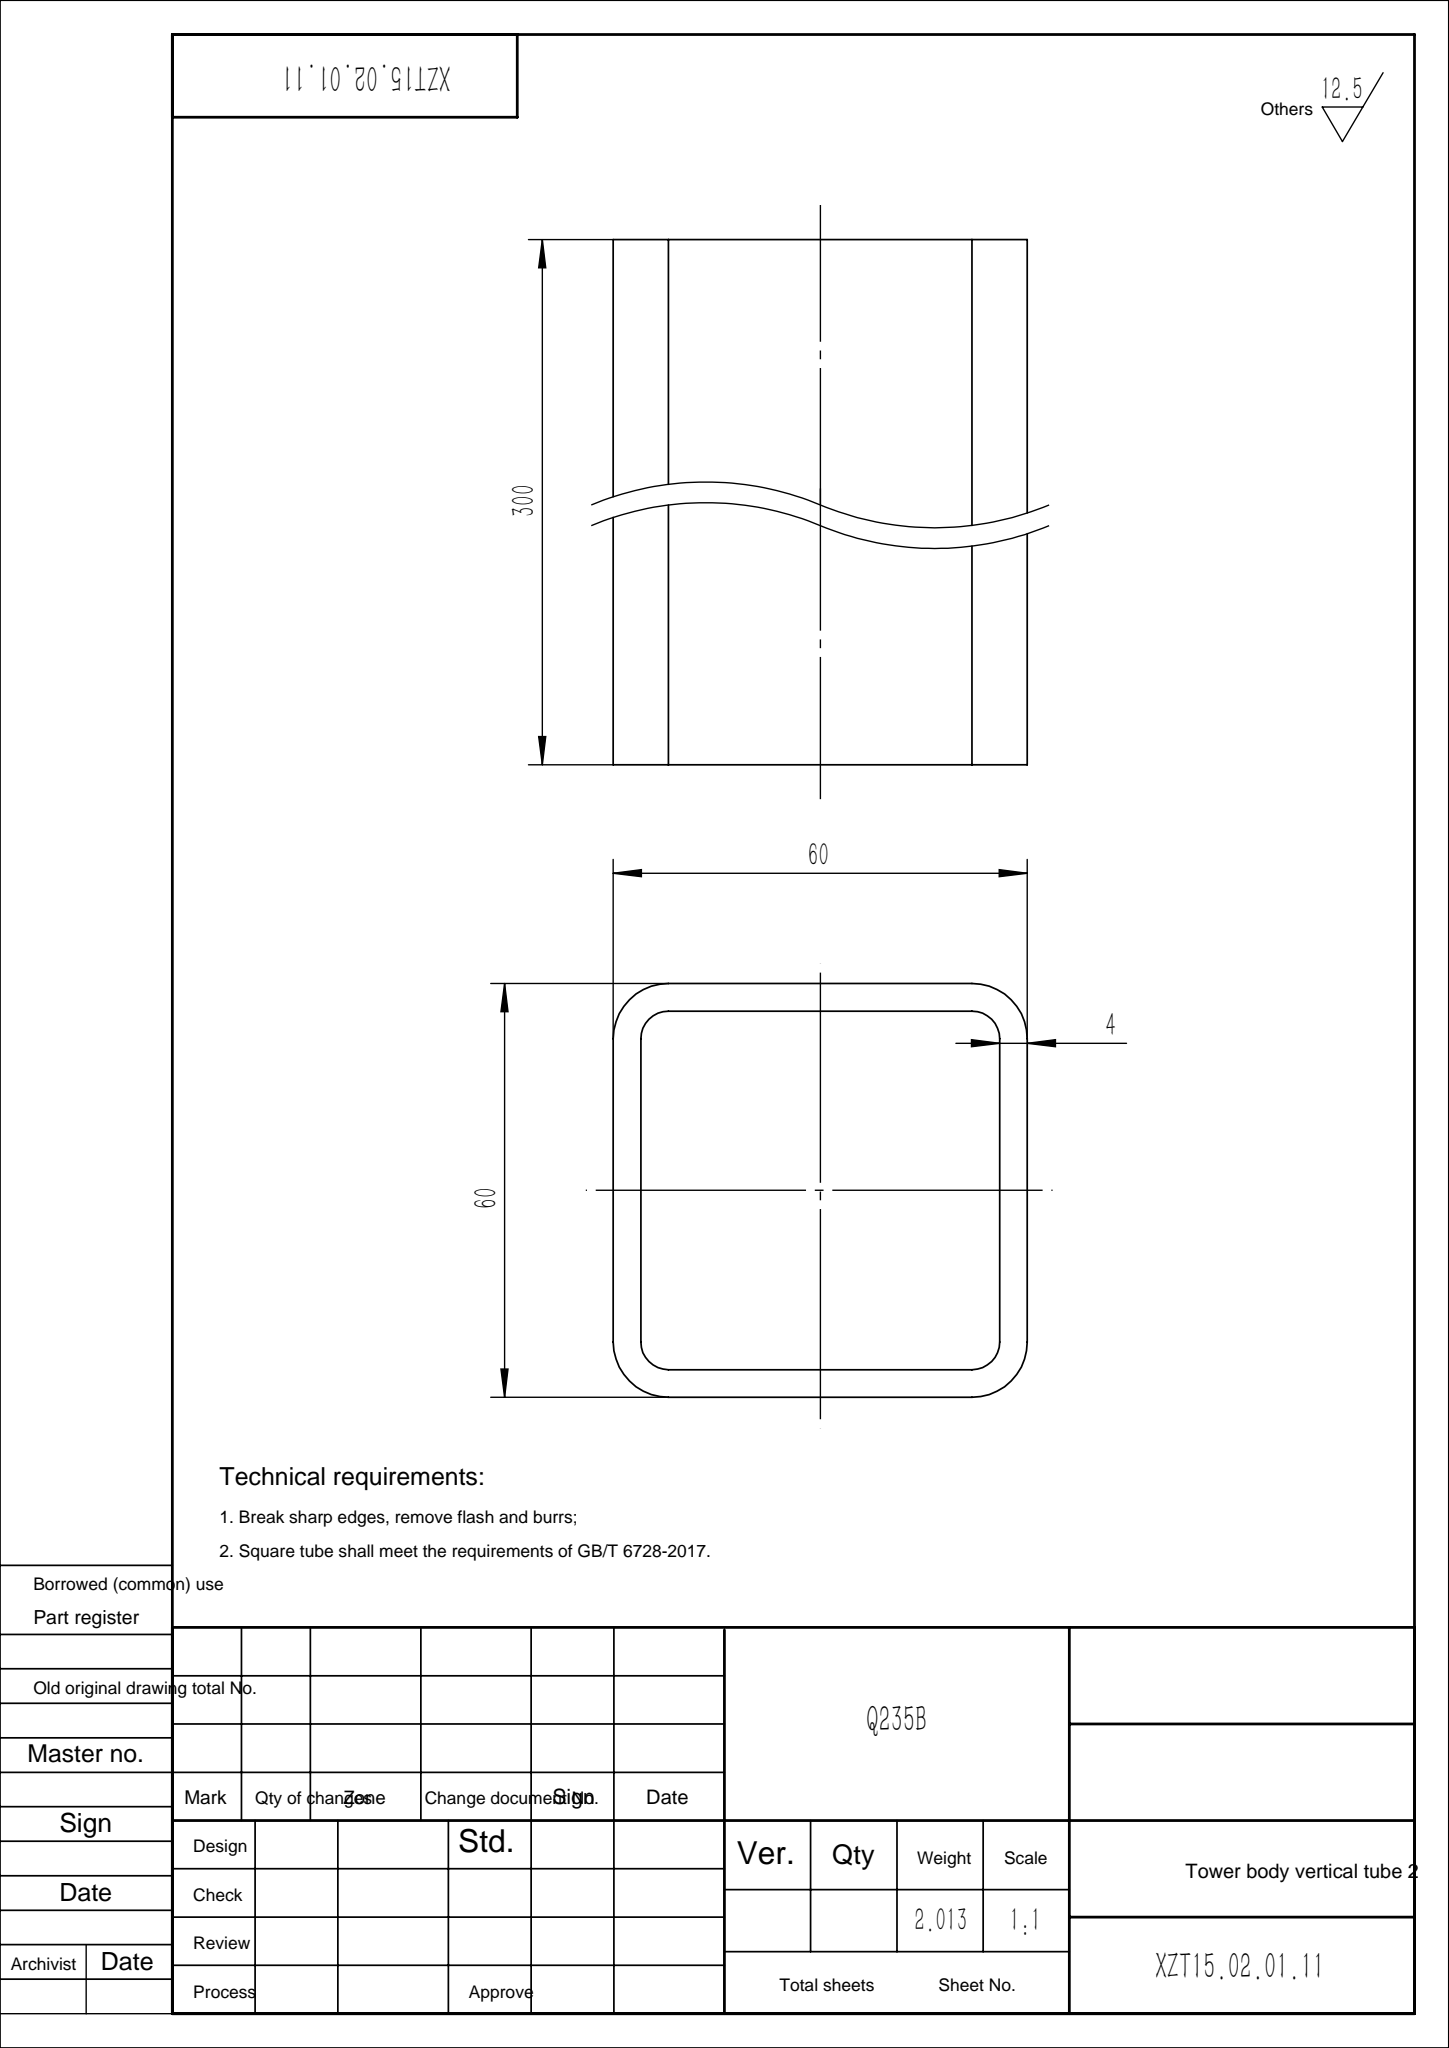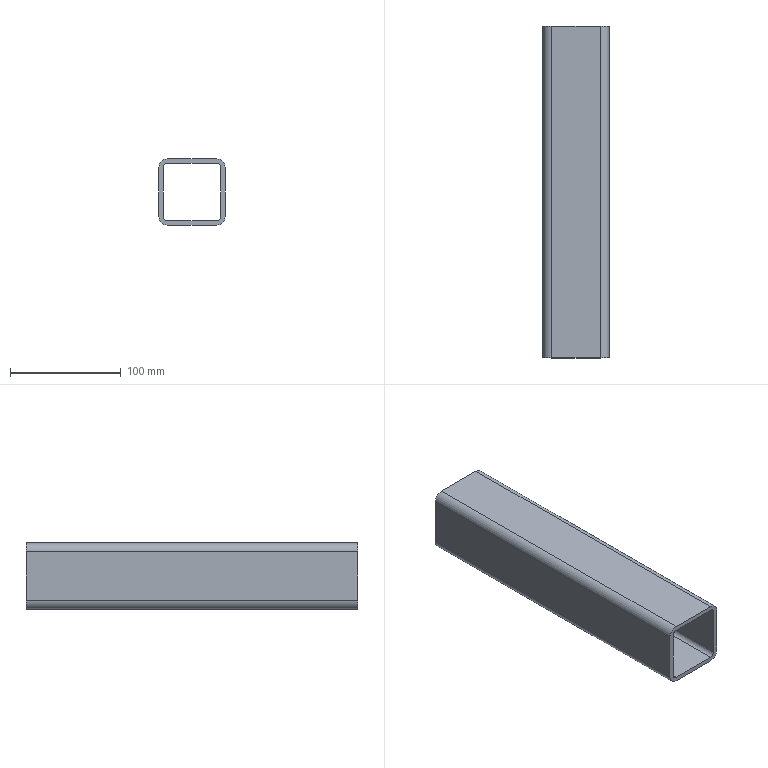Part | SolidWorks | features WeldMemberFeat 1, WeldmentFeature 1 | 1 solid | 18 faces | box 60 x 300 x 60 mm | volume 256439 mm3 | plane 10 | cylinder 8 | commonest cylinder face diameters 8 x4 16 x4
STEP:
#1=CARTESIAN_POINT('',(-30.,0.,22.));
#2=VERTEX_POINT('',#1);
#3=CARTESIAN_POINT('',(-22.,0.,30.));
#4=VERTEX_POINT('',#3);
#5=CARTESIAN_POINT('',(-22.,0.,22.));
#6=DIRECTION('',(0.,1.,0.));
#7=DIRECTION('',(0.,0.,1.));
#8=AXIS2_PLACEMENT_3D('',#5,#6,#7);
#9=CIRCLE('',#8,8.);
#10=EDGE_CURVE('',#2,#4,#9,.T.);
#11=ORIENTED_EDGE('',*,*,#10,.T.);
#12=CARTESIAN_POINT('',(-22.,300.,30.));
#13=VERTEX_POINT('',#12);
#14=CARTESIAN_POINT('',(-22.,300.,30.));
#15=DIRECTION('',(0.,-1.,0.));
#16=VECTOR('',#15,1000.);
#17=LINE('',#14,#16);
#18=EDGE_CURVE('',#13,#4,#17,.T.);
#19=ORIENTED_EDGE('',*,*,#18,.F.);
#20=CARTESIAN_POINT('',(-30.,300.,22.));
#21=VERTEX_POINT('',#20);
#22=CARTESIAN_POINT('',(-22.,300.,22.));
#23=DIRECTION('',(0.,1.,0.));
#24=DIRECTION('',(0.,0.,1.));
#25=AXIS2_PLACEMENT_3D('',#22,#23,#24);
#26=CIRCLE('',#25,8.);
#27=EDGE_CURVE('',#21,#13,#26,.T.);
#28=ORIENTED_EDGE('',*,*,#27,.F.);
#29=CARTESIAN_POINT('',(-30.,300.,22.));
#30=DIRECTION('',(0.,-1.,0.));
#31=VECTOR('',#30,1000.);
#32=LINE('',#29,#31);
#33=EDGE_CURVE('',#21,#2,#32,.T.);
#34=ORIENTED_EDGE('',*,*,#33,.T.);
#35=EDGE_LOOP('',(#11,#19,#28,#34));
#36=FACE_OUTER_BOUND('',#35,.T.);
#37=CARTESIAN_POINT('',(-22.,300.,22.));
#38=DIRECTION('',(0.,-1.,0.));
#39=DIRECTION('',(0.,0.,-1.));
#40=AXIS2_PLACEMENT_3D('',#37,#38,#39);
#41=CYLINDRICAL_SURFACE('',#40,8.);
#42=ADVANCED_FACE('',(#36),#41,.T.);
#43=CARTESIAN_POINT('',(22.,0.,30.));
#44=VERTEX_POINT('',#43);
#45=CARTESIAN_POINT('',(-22.,0.,30.));
#46=DIRECTION('',(1.,0.,0.));
#47=VECTOR('',#46,1000.);
#48=LINE('',#45,#47);
#49=EDGE_CURVE('',#4,#44,#48,.T.);
#50=ORIENTED_EDGE('',*,*,#49,.T.);
#51=CARTESIAN_POINT('',(22.,300.,30.));
#52=VERTEX_POINT('',#51);
#53=CARTESIAN_POINT('',(22.,300.,30.));
#54=DIRECTION('',(0.,-1.,0.));
#55=VECTOR('',#54,1000.);
#56=LINE('',#53,#55);
#57=EDGE_CURVE('',#52,#44,#56,.T.);
#58=ORIENTED_EDGE('',*,*,#57,.F.);
#59=CARTESIAN_POINT('',(-22.,300.,30.));
#60=DIRECTION('',(1.,0.,0.));
#61=VECTOR('',#60,1000.);
#62=LINE('',#59,#61);
#63=EDGE_CURVE('',#13,#52,#62,.T.);
#64=ORIENTED_EDGE('',*,*,#63,.F.);
#65=ORIENTED_EDGE('',*,*,#18,.T.);
#66=EDGE_LOOP('',(#50,#58,#64,#65));
#67=FACE_OUTER_BOUND('',#66,.T.);
#68=CARTESIAN_POINT('',(-22.,300.,30.));
#69=DIRECTION('',(0.,0.,-1.));
#70=DIRECTION('',(-1.,0.,0.));
#71=AXIS2_PLACEMENT_3D('',#68,#69,#70);
#72=PLANE('',#71);
#73=ADVANCED_FACE('',(#67),#72,.F.);
#74=CARTESIAN_POINT('',(30.,0.,22.));
#75=VERTEX_POINT('',#74);
#76=CARTESIAN_POINT('',(22.,0.,22.));
#77=DIRECTION('',(0.,1.,0.));
#78=DIRECTION('',(0.,0.,1.));
#79=AXIS2_PLACEMENT_3D('',#76,#77,#78);
#80=CIRCLE('',#79,8.);
#81=EDGE_CURVE('',#44,#75,#80,.T.);
#82=ORIENTED_EDGE('',*,*,#81,.T.);
#83=CARTESIAN_POINT('',(30.,300.,22.));
#84=VERTEX_POINT('',#83);
#85=CARTESIAN_POINT('',(30.,300.,22.));
#86=DIRECTION('',(0.,-1.,0.));
#87=VECTOR('',#86,1000.);
#88=LINE('',#85,#87);
#89=EDGE_CURVE('',#84,#75,#88,.T.);
#90=ORIENTED_EDGE('',*,*,#89,.F.);
#91=CARTESIAN_POINT('',(22.,300.,22.));
#92=DIRECTION('',(0.,1.,0.));
#93=DIRECTION('',(0.,0.,1.));
#94=AXIS2_PLACEMENT_3D('',#91,#92,#93);
#95=CIRCLE('',#94,8.);
#96=EDGE_CURVE('',#52,#84,#95,.T.);
#97=ORIENTED_EDGE('',*,*,#96,.F.);
#98=ORIENTED_EDGE('',*,*,#57,.T.);
#99=EDGE_LOOP('',(#82,#90,#97,#98));
#100=FACE_OUTER_BOUND('',#99,.T.);
#101=CARTESIAN_POINT('',(22.,300.,22.));
#102=DIRECTION('',(0.,-1.,0.));
#103=DIRECTION('',(0.,0.,-1.));
#104=AXIS2_PLACEMENT_3D('',#101,#102,#103);
#105=CYLINDRICAL_SURFACE('',#104,8.);
#106=ADVANCED_FACE('',(#100),#105,.T.);
#107=CARTESIAN_POINT('',(30.,0.,-22.));
#108=VERTEX_POINT('',#107);
#109=CARTESIAN_POINT('',(30.,0.,-22.));
#110=DIRECTION('',(0.,0.,-1.));
#111=VECTOR('',#110,1000.);
#112=LINE('',#109,#111);
#113=EDGE_CURVE('',#75,#108,#112,.T.);
#114=ORIENTED_EDGE('',*,*,#113,.T.);
#115=CARTESIAN_POINT('',(30.,300.,-22.));
#116=VERTEX_POINT('',#115);
#117=CARTESIAN_POINT('',(30.,300.,-22.));
#118=DIRECTION('',(0.,-1.,0.));
#119=VECTOR('',#118,1000.);
#120=LINE('',#117,#119);
#121=EDGE_CURVE('',#116,#108,#120,.T.);
#122=ORIENTED_EDGE('',*,*,#121,.F.);
#123=CARTESIAN_POINT('',(30.,300.,-22.));
#124=DIRECTION('',(0.,0.,-1.));
#125=VECTOR('',#124,1000.);
#126=LINE('',#123,#125);
#127=EDGE_CURVE('',#84,#116,#126,.T.);
#128=ORIENTED_EDGE('',*,*,#127,.F.);
#129=ORIENTED_EDGE('',*,*,#89,.T.);
#130=EDGE_LOOP('',(#114,#122,#128,#129));
#131=FACE_OUTER_BOUND('',#130,.T.);
#132=CARTESIAN_POINT('',(30.,300.,-22.));
#133=DIRECTION('',(-1.,0.,0.));
#134=DIRECTION('',(0.,0.,1.));
#135=AXIS2_PLACEMENT_3D('',#132,#133,#134);
#136=PLANE('',#135);
#137=ADVANCED_FACE('',(#131),#136,.F.);
#138=CARTESIAN_POINT('',(22.,0.,-30.));
#139=VERTEX_POINT('',#138);
#140=CARTESIAN_POINT('',(22.,0.,-22.));
#141=DIRECTION('',(0.,1.,0.));
#142=DIRECTION('',(0.,0.,1.));
#143=AXIS2_PLACEMENT_3D('',#140,#141,#142);
#144=CIRCLE('',#143,8.);
#145=EDGE_CURVE('',#108,#139,#144,.T.);
#146=ORIENTED_EDGE('',*,*,#145,.T.);
#147=CARTESIAN_POINT('',(22.,300.,-30.));
#148=VERTEX_POINT('',#147);
#149=CARTESIAN_POINT('',(22.,300.,-30.));
#150=DIRECTION('',(0.,-1.,0.));
#151=VECTOR('',#150,1000.);
#152=LINE('',#149,#151);
#153=EDGE_CURVE('',#148,#139,#152,.T.);
#154=ORIENTED_EDGE('',*,*,#153,.F.);
#155=CARTESIAN_POINT('',(22.,300.,-22.));
#156=DIRECTION('',(0.,1.,0.));
#157=DIRECTION('',(0.,0.,1.));
#158=AXIS2_PLACEMENT_3D('',#155,#156,#157);
#159=CIRCLE('',#158,8.);
#160=EDGE_CURVE('',#116,#148,#159,.T.);
#161=ORIENTED_EDGE('',*,*,#160,.F.);
#162=ORIENTED_EDGE('',*,*,#121,.T.);
#163=EDGE_LOOP('',(#146,#154,#161,#162));
#164=FACE_OUTER_BOUND('',#163,.T.);
#165=CARTESIAN_POINT('',(22.,300.,-22.));
#166=DIRECTION('',(0.,-1.,0.));
#167=DIRECTION('',(0.,0.,-1.));
#168=AXIS2_PLACEMENT_3D('',#165,#166,#167);
#169=CYLINDRICAL_SURFACE('',#168,8.);
#170=ADVANCED_FACE('',(#164),#169,.T.);
#171=CARTESIAN_POINT('',(-22.,0.,-30.));
#172=VERTEX_POINT('',#171);
#173=CARTESIAN_POINT('',(22.,0.,-30.));
#174=DIRECTION('',(-1.,0.,0.));
#175=VECTOR('',#174,1000.);
#176=LINE('',#173,#175);
#177=EDGE_CURVE('',#139,#172,#176,.T.);
#178=ORIENTED_EDGE('',*,*,#177,.T.);
#179=CARTESIAN_POINT('',(-22.,300.,-30.));
#180=VERTEX_POINT('',#179);
#181=CARTESIAN_POINT('',(-22.,300.,-30.));
#182=DIRECTION('',(0.,-1.,0.));
#183=VECTOR('',#182,1000.);
#184=LINE('',#181,#183);
#185=EDGE_CURVE('',#180,#172,#184,.T.);
#186=ORIENTED_EDGE('',*,*,#185,.F.);
#187=CARTESIAN_POINT('',(22.,300.,-30.));
#188=DIRECTION('',(-1.,0.,0.));
#189=VECTOR('',#188,1000.);
#190=LINE('',#187,#189);
#191=EDGE_CURVE('',#148,#180,#190,.T.);
#192=ORIENTED_EDGE('',*,*,#191,.F.);
#193=ORIENTED_EDGE('',*,*,#153,.T.);
#194=EDGE_LOOP('',(#178,#186,#192,#193));
#195=FACE_OUTER_BOUND('',#194,.T.);
#196=CARTESIAN_POINT('',(22.,300.,-30.));
#197=DIRECTION('',(0.,0.,1.));
#198=DIRECTION('',(1.,0.,0.));
#199=AXIS2_PLACEMENT_3D('',#196,#197,#198);
#200=PLANE('',#199);
#201=ADVANCED_FACE('',(#195),#200,.F.);
#202=CARTESIAN_POINT('',(-30.,0.,-22.));
#203=VERTEX_POINT('',#202);
#204=CARTESIAN_POINT('',(-22.,0.,-22.));
#205=DIRECTION('',(0.,1.,0.));
#206=DIRECTION('',(0.,0.,1.));
#207=AXIS2_PLACEMENT_3D('',#204,#205,#206);
#208=CIRCLE('',#207,8.);
#209=EDGE_CURVE('',#172,#203,#208,.T.);
#210=ORIENTED_EDGE('',*,*,#209,.T.);
#211=CARTESIAN_POINT('',(-30.,300.,-22.));
#212=VERTEX_POINT('',#211);
#213=CARTESIAN_POINT('',(-30.,300.,-22.));
#214=DIRECTION('',(0.,-1.,0.));
#215=VECTOR('',#214,1000.);
#216=LINE('',#213,#215);
#217=EDGE_CURVE('',#212,#203,#216,.T.);
#218=ORIENTED_EDGE('',*,*,#217,.F.);
#219=CARTESIAN_POINT('',(-22.,300.,-22.));
#220=DIRECTION('',(0.,1.,0.));
#221=DIRECTION('',(0.,0.,1.));
#222=AXIS2_PLACEMENT_3D('',#219,#220,#221);
#223=CIRCLE('',#222,8.);
#224=EDGE_CURVE('',#180,#212,#223,.T.);
#225=ORIENTED_EDGE('',*,*,#224,.F.);
#226=ORIENTED_EDGE('',*,*,#185,.T.);
#227=EDGE_LOOP('',(#210,#218,#225,#226));
#228=FACE_OUTER_BOUND('',#227,.T.);
#229=CARTESIAN_POINT('',(-22.,300.,-22.));
#230=DIRECTION('',(0.,-1.,0.));
#231=DIRECTION('',(0.,0.,-1.));
#232=AXIS2_PLACEMENT_3D('',#229,#230,#231);
#233=CYLINDRICAL_SURFACE('',#232,8.);
#234=ADVANCED_FACE('',(#228),#233,.T.);
#235=CARTESIAN_POINT('',(22.,0.,26.));
#236=VERTEX_POINT('',#235);
#237=CARTESIAN_POINT('',(26.,0.,22.));
#238=VERTEX_POINT('',#237);
#239=CARTESIAN_POINT('',(22.,0.,22.));
#240=DIRECTION('',(0.,1.,0.));
#241=DIRECTION('',(0.,0.,1.));
#242=AXIS2_PLACEMENT_3D('',#239,#240,#241);
#243=CIRCLE('',#242,4.);
#244=EDGE_CURVE('',#236,#238,#243,.T.);
#245=ORIENTED_EDGE('',*,*,#244,.F.);
#246=CARTESIAN_POINT('',(22.,300.,26.));
#247=VERTEX_POINT('',#246);
#248=CARTESIAN_POINT('',(22.,300.,26.));
#249=DIRECTION('',(0.,-1.,0.));
#250=VECTOR('',#249,1000.);
#251=LINE('',#248,#250);
#252=EDGE_CURVE('',#247,#236,#251,.T.);
#253=ORIENTED_EDGE('',*,*,#252,.F.);
#254=CARTESIAN_POINT('',(26.,300.,22.));
#255=VERTEX_POINT('',#254);
#256=CARTESIAN_POINT('',(22.,300.,22.));
#257=DIRECTION('',(0.,1.,0.));
#258=DIRECTION('',(0.,0.,1.));
#259=AXIS2_PLACEMENT_3D('',#256,#257,#258);
#260=CIRCLE('',#259,4.);
#261=EDGE_CURVE('',#247,#255,#260,.T.);
#262=ORIENTED_EDGE('',*,*,#261,.T.);
#263=CARTESIAN_POINT('',(26.,300.,22.));
#264=DIRECTION('',(0.,-1.,0.));
#265=VECTOR('',#264,1000.);
#266=LINE('',#263,#265);
#267=EDGE_CURVE('',#255,#238,#266,.T.);
#268=ORIENTED_EDGE('',*,*,#267,.T.);
#269=EDGE_LOOP('',(#245,#253,#262,#268));
#270=FACE_OUTER_BOUND('',#269,.T.);
#271=CARTESIAN_POINT('',(22.,300.,22.));
#272=DIRECTION('',(0.,-1.,0.));
#273=DIRECTION('',(0.,0.,-1.));
#274=AXIS2_PLACEMENT_3D('',#271,#272,#273);
#275=CYLINDRICAL_SURFACE('',#274,4.);
#276=ADVANCED_FACE('',(#270),#275,.F.);
#277=CARTESIAN_POINT('',(-22.,0.,26.));
#278=VERTEX_POINT('',#277);
#279=CARTESIAN_POINT('',(-22.,0.,26.));
#280=DIRECTION('',(1.,0.,0.));
#281=VECTOR('',#280,1000.);
#282=LINE('',#279,#281);
#283=EDGE_CURVE('',#278,#236,#282,.T.);
#284=ORIENTED_EDGE('',*,*,#283,.F.);
#285=CARTESIAN_POINT('',(-22.,300.,26.));
#286=VERTEX_POINT('',#285);
#287=CARTESIAN_POINT('',(-22.,300.,26.));
#288=DIRECTION('',(0.,-1.,0.));
#289=VECTOR('',#288,1000.);
#290=LINE('',#287,#289);
#291=EDGE_CURVE('',#286,#278,#290,.T.);
#292=ORIENTED_EDGE('',*,*,#291,.F.);
#293=CARTESIAN_POINT('',(-22.,300.,26.));
#294=DIRECTION('',(1.,0.,0.));
#295=VECTOR('',#294,1000.);
#296=LINE('',#293,#295);
#297=EDGE_CURVE('',#286,#247,#296,.T.);
#298=ORIENTED_EDGE('',*,*,#297,.T.);
#299=ORIENTED_EDGE('',*,*,#252,.T.);
#300=EDGE_LOOP('',(#284,#292,#298,#299));
#301=FACE_OUTER_BOUND('',#300,.T.);
#302=CARTESIAN_POINT('',(-22.,300.,26.));
#303=DIRECTION('',(0.,0.,-1.));
#304=DIRECTION('',(-1.,0.,0.));
#305=AXIS2_PLACEMENT_3D('',#302,#303,#304);
#306=PLANE('',#305);
#307=ADVANCED_FACE('',(#301),#306,.T.);
#308=CARTESIAN_POINT('',(-26.,0.,22.));
#309=VERTEX_POINT('',#308);
#310=CARTESIAN_POINT('',(-22.,0.,22.));
#311=DIRECTION('',(0.,1.,0.));
#312=DIRECTION('',(0.,0.,1.));
#313=AXIS2_PLACEMENT_3D('',#310,#311,#312);
#314=CIRCLE('',#313,4.);
#315=EDGE_CURVE('',#309,#278,#314,.T.);
#316=ORIENTED_EDGE('',*,*,#315,.F.);
#317=CARTESIAN_POINT('',(-26.,300.,22.));
#318=VERTEX_POINT('',#317);
#319=CARTESIAN_POINT('',(-26.,300.,22.));
#320=DIRECTION('',(0.,-1.,0.));
#321=VECTOR('',#320,1000.);
#322=LINE('',#319,#321);
#323=EDGE_CURVE('',#318,#309,#322,.T.);
#324=ORIENTED_EDGE('',*,*,#323,.F.);
#325=CARTESIAN_POINT('',(-22.,300.,22.));
#326=DIRECTION('',(0.,1.,0.));
#327=DIRECTION('',(0.,0.,1.));
#328=AXIS2_PLACEMENT_3D('',#325,#326,#327);
#329=CIRCLE('',#328,4.);
#330=EDGE_CURVE('',#318,#286,#329,.T.);
#331=ORIENTED_EDGE('',*,*,#330,.T.);
#332=ORIENTED_EDGE('',*,*,#291,.T.);
#333=EDGE_LOOP('',(#316,#324,#331,#332));
#334=FACE_OUTER_BOUND('',#333,.T.);
#335=CARTESIAN_POINT('',(-22.,300.,22.));
#336=DIRECTION('',(0.,-1.,0.));
#337=DIRECTION('',(0.,0.,-1.));
#338=AXIS2_PLACEMENT_3D('',#335,#336,#337);
#339=CYLINDRICAL_SURFACE('',#338,4.);
#340=ADVANCED_FACE('',(#334),#339,.F.);
#341=CARTESIAN_POINT('',(-26.,0.,-22.));
#342=VERTEX_POINT('',#341);
#343=CARTESIAN_POINT('',(-26.,0.,22.));
#344=DIRECTION('',(0.,0.,1.));
#345=VECTOR('',#344,1000.);
#346=LINE('',#343,#345);
#347=EDGE_CURVE('',#342,#309,#346,.T.);
#348=ORIENTED_EDGE('',*,*,#347,.F.);
#349=CARTESIAN_POINT('',(-26.,300.,-22.));
#350=VERTEX_POINT('',#349);
#351=CARTESIAN_POINT('',(-26.,300.,-22.));
#352=DIRECTION('',(0.,-1.,0.));
#353=VECTOR('',#352,1000.);
#354=LINE('',#351,#353);
#355=EDGE_CURVE('',#350,#342,#354,.T.);
#356=ORIENTED_EDGE('',*,*,#355,.F.);
#357=CARTESIAN_POINT('',(-26.,300.,22.));
#358=DIRECTION('',(0.,0.,1.));
#359=VECTOR('',#358,1000.);
#360=LINE('',#357,#359);
#361=EDGE_CURVE('',#350,#318,#360,.T.);
#362=ORIENTED_EDGE('',*,*,#361,.T.);
#363=ORIENTED_EDGE('',*,*,#323,.T.);
#364=EDGE_LOOP('',(#348,#356,#362,#363));
#365=FACE_OUTER_BOUND('',#364,.T.);
#366=CARTESIAN_POINT('',(-26.,300.,22.));
#367=DIRECTION('',(1.,0.,0.));
#368=DIRECTION('',(0.,0.,-1.));
#369=AXIS2_PLACEMENT_3D('',#366,#367,#368);
#370=PLANE('',#369);
#371=ADVANCED_FACE('',(#365),#370,.T.);
#372=CARTESIAN_POINT('',(-22.,0.,-26.));
#373=VERTEX_POINT('',#372);
#374=CARTESIAN_POINT('',(-22.,0.,-22.));
#375=DIRECTION('',(0.,1.,0.));
#376=DIRECTION('',(0.,0.,1.));
#377=AXIS2_PLACEMENT_3D('',#374,#375,#376);
#378=CIRCLE('',#377,4.);
#379=EDGE_CURVE('',#373,#342,#378,.T.);
#380=ORIENTED_EDGE('',*,*,#379,.F.);
#381=CARTESIAN_POINT('',(-22.,300.,-26.));
#382=VERTEX_POINT('',#381);
#383=CARTESIAN_POINT('',(-22.,300.,-26.));
#384=DIRECTION('',(0.,-1.,0.));
#385=VECTOR('',#384,1000.);
#386=LINE('',#383,#385);
#387=EDGE_CURVE('',#382,#373,#386,.T.);
#388=ORIENTED_EDGE('',*,*,#387,.F.);
#389=CARTESIAN_POINT('',(-22.,300.,-22.));
#390=DIRECTION('',(0.,1.,0.));
#391=DIRECTION('',(0.,0.,1.));
#392=AXIS2_PLACEMENT_3D('',#389,#390,#391);
#393=CIRCLE('',#392,4.);
#394=EDGE_CURVE('',#382,#350,#393,.T.);
#395=ORIENTED_EDGE('',*,*,#394,.T.);
#396=ORIENTED_EDGE('',*,*,#355,.T.);
#397=EDGE_LOOP('',(#380,#388,#395,#396));
#398=FACE_OUTER_BOUND('',#397,.T.);
#399=CARTESIAN_POINT('',(-22.,300.,-22.));
#400=DIRECTION('',(0.,-1.,0.));
#401=DIRECTION('',(0.,0.,-1.));
#402=AXIS2_PLACEMENT_3D('',#399,#400,#401);
#403=CYLINDRICAL_SURFACE('',#402,4.);
#404=ADVANCED_FACE('',(#398),#403,.F.);
#405=CARTESIAN_POINT('',(22.,0.,-26.));
#406=VERTEX_POINT('',#405);
#407=CARTESIAN_POINT('',(22.,0.,-26.));
#408=DIRECTION('',(-1.,0.,0.));
#409=VECTOR('',#408,1000.);
#410=LINE('',#407,#409);
#411=EDGE_CURVE('',#406,#373,#410,.T.);
#412=ORIENTED_EDGE('',*,*,#411,.F.);
#413=CARTESIAN_POINT('',(22.,300.,-26.));
#414=VERTEX_POINT('',#413);
#415=CARTESIAN_POINT('',(22.,300.,-26.));
#416=DIRECTION('',(0.,-1.,0.));
#417=VECTOR('',#416,1000.);
#418=LINE('',#415,#417);
#419=EDGE_CURVE('',#414,#406,#418,.T.);
#420=ORIENTED_EDGE('',*,*,#419,.F.);
#421=CARTESIAN_POINT('',(22.,300.,-26.));
#422=DIRECTION('',(-1.,0.,0.));
#423=VECTOR('',#422,1000.);
#424=LINE('',#421,#423);
#425=EDGE_CURVE('',#414,#382,#424,.T.);
#426=ORIENTED_EDGE('',*,*,#425,.T.);
#427=ORIENTED_EDGE('',*,*,#387,.T.);
#428=EDGE_LOOP('',(#412,#420,#426,#427));
#429=FACE_OUTER_BOUND('',#428,.T.);
#430=CARTESIAN_POINT('',(22.,300.,-26.));
#431=DIRECTION('',(0.,0.,1.));
#432=DIRECTION('',(1.,0.,0.));
#433=AXIS2_PLACEMENT_3D('',#430,#431,#432);
#434=PLANE('',#433);
#435=ADVANCED_FACE('',(#429),#434,.T.);
#436=CARTESIAN_POINT('',(26.,0.,-22.));
#437=VERTEX_POINT('',#436);
#438=CARTESIAN_POINT('',(22.,0.,-22.));
#439=DIRECTION('',(0.,1.,0.));
#440=DIRECTION('',(0.,0.,1.));
#441=AXIS2_PLACEMENT_3D('',#438,#439,#440);
#442=CIRCLE('',#441,4.);
#443=EDGE_CURVE('',#437,#406,#442,.T.);
#444=ORIENTED_EDGE('',*,*,#443,.F.);
#445=CARTESIAN_POINT('',(26.,300.,-22.));
#446=VERTEX_POINT('',#445);
#447=CARTESIAN_POINT('',(26.,300.,-22.));
#448=DIRECTION('',(0.,-1.,0.));
#449=VECTOR('',#448,1000.);
#450=LINE('',#447,#449);
#451=EDGE_CURVE('',#446,#437,#450,.T.);
#452=ORIENTED_EDGE('',*,*,#451,.F.);
#453=CARTESIAN_POINT('',(22.,300.,-22.));
#454=DIRECTION('',(0.,1.,0.));
#455=DIRECTION('',(0.,0.,1.));
#456=AXIS2_PLACEMENT_3D('',#453,#454,#455);
#457=CIRCLE('',#456,4.);
#458=EDGE_CURVE('',#446,#414,#457,.T.);
#459=ORIENTED_EDGE('',*,*,#458,.T.);
#460=ORIENTED_EDGE('',*,*,#419,.T.);
#461=EDGE_LOOP('',(#444,#452,#459,#460));
#462=FACE_OUTER_BOUND('',#461,.T.);
#463=CARTESIAN_POINT('',(22.,300.,-22.));
#464=DIRECTION('',(0.,-1.,0.));
#465=DIRECTION('',(0.,0.,-1.));
#466=AXIS2_PLACEMENT_3D('',#463,#464,#465);
#467=CYLINDRICAL_SURFACE('',#466,4.);
#468=ADVANCED_FACE('',(#462),#467,.F.);
#469=CARTESIAN_POINT('',(26.,0.,-22.));
#470=DIRECTION('',(0.,0.,-1.));
#471=VECTOR('',#470,1000.);
#472=LINE('',#469,#471);
#473=EDGE_CURVE('',#238,#437,#472,.T.);
#474=ORIENTED_EDGE('',*,*,#473,.F.);
#475=ORIENTED_EDGE('',*,*,#267,.F.);
#476=CARTESIAN_POINT('',(26.,300.,-22.));
#477=DIRECTION('',(0.,0.,-1.));
#478=VECTOR('',#477,1000.);
#479=LINE('',#476,#478);
#480=EDGE_CURVE('',#255,#446,#479,.T.);
#481=ORIENTED_EDGE('',*,*,#480,.T.);
#482=ORIENTED_EDGE('',*,*,#451,.T.);
#483=EDGE_LOOP('',(#474,#475,#481,#482));
#484=FACE_OUTER_BOUND('',#483,.T.);
#485=CARTESIAN_POINT('',(26.,300.,-22.));
#486=DIRECTION('',(-1.,0.,0.));
#487=DIRECTION('',(0.,0.,1.));
#488=AXIS2_PLACEMENT_3D('',#485,#486,#487);
#489=PLANE('',#488);
#490=ADVANCED_FACE('',(#484),#489,.T.);
#491=CARTESIAN_POINT('',(-30.,0.,22.));
#492=DIRECTION('',(0.,0.,1.));
#493=VECTOR('',#492,1000.);
#494=LINE('',#491,#493);
#495=EDGE_CURVE('',#203,#2,#494,.T.);
#496=ORIENTED_EDGE('',*,*,#495,.T.);
#497=ORIENTED_EDGE('',*,*,#33,.F.);
#498=CARTESIAN_POINT('',(-30.,300.,22.));
#499=DIRECTION('',(0.,0.,1.));
#500=VECTOR('',#499,1000.);
#501=LINE('',#498,#500);
#502=EDGE_CURVE('',#212,#21,#501,.T.);
#503=ORIENTED_EDGE('',*,*,#502,.F.);
#504=ORIENTED_EDGE('',*,*,#217,.T.);
#505=EDGE_LOOP('',(#496,#497,#503,#504));
#506=FACE_OUTER_BOUND('',#505,.T.);
#507=CARTESIAN_POINT('',(-30.,300.,22.));
#508=DIRECTION('',(1.,0.,0.));
#509=DIRECTION('',(0.,0.,-1.));
#510=AXIS2_PLACEMENT_3D('',#507,#508,#509);
#511=PLANE('',#510);
#512=ADVANCED_FACE('',(#506),#511,.F.);
#513=ORIENTED_EDGE('',*,*,#261,.F.);
#514=ORIENTED_EDGE('',*,*,#297,.F.);
#515=ORIENTED_EDGE('',*,*,#330,.F.);
#516=ORIENTED_EDGE('',*,*,#361,.F.);
#517=ORIENTED_EDGE('',*,*,#394,.F.);
#518=ORIENTED_EDGE('',*,*,#425,.F.);
#519=ORIENTED_EDGE('',*,*,#458,.F.);
#520=ORIENTED_EDGE('',*,*,#480,.F.);
#521=EDGE_LOOP('',(#513,#514,#515,#516,#517,#518,#519,#520));
#522=FACE_BOUND('',#521,.T.);
#523=ORIENTED_EDGE('',*,*,#27,.T.);
#524=ORIENTED_EDGE('',*,*,#63,.T.);
#525=ORIENTED_EDGE('',*,*,#96,.T.);
#526=ORIENTED_EDGE('',*,*,#127,.T.);
#527=ORIENTED_EDGE('',*,*,#160,.T.);
#528=ORIENTED_EDGE('',*,*,#191,.T.);
#529=ORIENTED_EDGE('',*,*,#224,.T.);
#530=ORIENTED_EDGE('',*,*,#502,.T.);
#531=EDGE_LOOP('',(#523,#524,#525,#526,#527,#528,#529,#530));
#532=FACE_OUTER_BOUND('',#531,.T.);
#533=CARTESIAN_POINT('',(-22.,300.,22.));
#534=DIRECTION('',(0.,1.,0.));
#535=DIRECTION('',(0.,0.,1.));
#536=AXIS2_PLACEMENT_3D('',#533,#534,#535);
#537=PLANE('',#536);
#538=ADVANCED_FACE('',(#522,#532),#537,.T.);
#539=ORIENTED_EDGE('',*,*,#244,.T.);
#540=ORIENTED_EDGE('',*,*,#473,.T.);
#541=ORIENTED_EDGE('',*,*,#443,.T.);
#542=ORIENTED_EDGE('',*,*,#411,.T.);
#543=ORIENTED_EDGE('',*,*,#379,.T.);
#544=ORIENTED_EDGE('',*,*,#347,.T.);
#545=ORIENTED_EDGE('',*,*,#315,.T.);
#546=ORIENTED_EDGE('',*,*,#283,.T.);
#547=EDGE_LOOP('',(#539,#540,#541,#542,#543,#544,#545,#546));
#548=FACE_BOUND('',#547,.T.);
#549=ORIENTED_EDGE('',*,*,#10,.F.);
#550=ORIENTED_EDGE('',*,*,#495,.F.);
#551=ORIENTED_EDGE('',*,*,#209,.F.);
#552=ORIENTED_EDGE('',*,*,#177,.F.);
#553=ORIENTED_EDGE('',*,*,#145,.F.);
#554=ORIENTED_EDGE('',*,*,#113,.F.);
#555=ORIENTED_EDGE('',*,*,#81,.F.);
#556=ORIENTED_EDGE('',*,*,#49,.F.);
#557=EDGE_LOOP('',(#549,#550,#551,#552,#553,#554,#555,#556));
#558=FACE_OUTER_BOUND('',#557,.T.);
#559=CARTESIAN_POINT('',(-22.,0.,22.));
#560=DIRECTION('',(0.,1.,0.));
#561=DIRECTION('',(0.,0.,1.));
#562=AXIS2_PLACEMENT_3D('',#559,#560,#561);
#563=PLANE('',#562);
#564=ADVANCED_FACE('',(#548,#558),#563,.F.);
#565=CLOSED_SHELL('',(#42,#73,#106,#137,#170,#201,#234,#276,#307,#340,#371,#404,#435,#468,#490,#512,#538,#564));
#566=MANIFOLD_SOLID_BREP('',#565);
#567=CARTESIAN_POINT('',(0.,0.,0.));
#568=DIRECTION('',(0.,0.,1.));
#569=DIRECTION('',(1.,0.,0.));
#570=AXIS2_PLACEMENT_3D('',#567,#568,#569);
#571=(LENGTH_UNIT()NAMED_UNIT(*)SI_UNIT(.MILLI.,.METRE.));
#572=UNCERTAINTY_MEASURE_WITH_UNIT(LENGTH_MEASURE(0.00001),#571,'','');
#573=(NAMED_UNIT(*)PLANE_ANGLE_UNIT()SI_UNIT($,.RADIAN.));
#574=(NAMED_UNIT(*)SI_UNIT($,.STERADIAN.)SOLID_ANGLE_UNIT());
#575=(GEOMETRIC_REPRESENTATION_CONTEXT(3)GLOBAL_UNCERTAINTY_ASSIGNED_CONTEXT((#572))GLOBAL_UNIT_ASSIGNED_CONTEXT((#571,#573,#574))REPRESENTATION_CONTEXT('',''));
#576=ADVANCED_BREP_SHAPE_REPRESENTATION('',(#566,#570),#575);